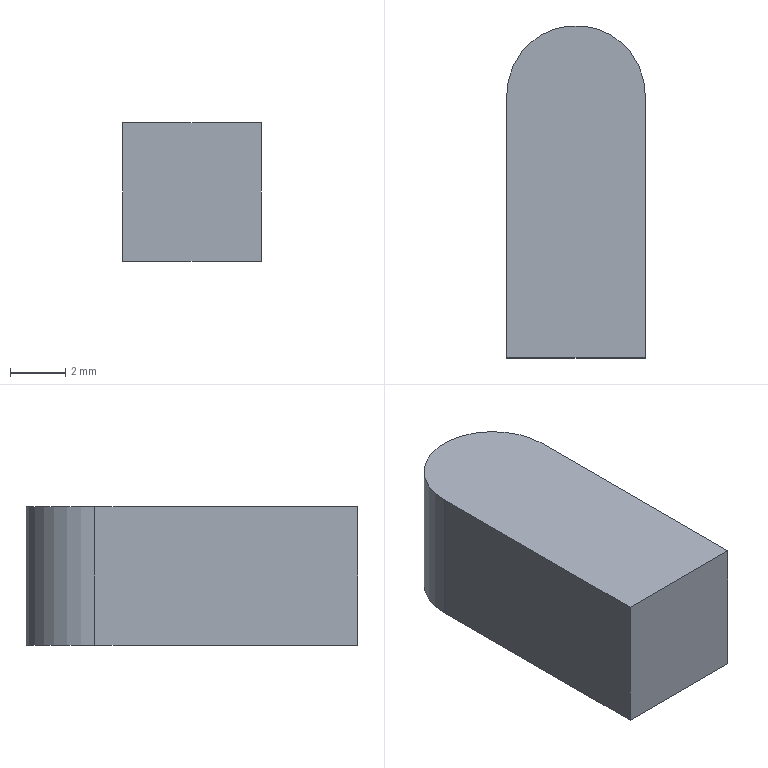Part | NX | features DATUM_CSYS 2, EXTRUDE 1, FACE_BLEND 1, SKETCH 1 | 1 solid | 6 faces | box 5 x 12 x 5 mm | volume 286.587 mm3 | plane 5 | cylinder 1 | commonest cylinder face diameters 5 x1
STEP:
#1=CARTESIAN_POINT('',(2.5,9.5,0.));
#2=VERTEX_POINT('',#1);
#3=CARTESIAN_POINT('',(2.5,9.5,5.));
#4=VERTEX_POINT('',#3);
#5=CARTESIAN_POINT('',(2.5,9.5,5.));
#6=DIRECTION('',(0.,0.,1.));
#7=VECTOR('',#6,1000.);
#8=LINE('',#5,#7);
#9=EDGE_CURVE('',#2,#4,#8,.T.);
#10=ORIENTED_EDGE('',*,*,#9,.F.);
#11=CARTESIAN_POINT('',(-2.5,9.5,0.));
#12=VERTEX_POINT('',#11);
#13=CARTESIAN_POINT('',(0.,9.5,0.));
#14=DIRECTION('',(0.,0.,1.));
#15=DIRECTION('',(1.,0.,0.));
#16=AXIS2_PLACEMENT_3D('',#13,#14,#15);
#17=CIRCLE('',#16,2.5);
#18=EDGE_CURVE('',#12,#2,#17,.F.);
#19=ORIENTED_EDGE('',*,*,#18,.F.);
#20=CARTESIAN_POINT('',(-2.5,9.5,5.));
#21=VERTEX_POINT('',#20);
#22=CARTESIAN_POINT('',(-2.5,9.5,5.));
#23=DIRECTION('',(0.,0.,1.));
#24=VECTOR('',#23,1000.);
#25=LINE('',#22,#24);
#26=EDGE_CURVE('',#21,#12,#25,.F.);
#27=ORIENTED_EDGE('',*,*,#26,.F.);
#28=CARTESIAN_POINT('',(0.,9.5,5.));
#29=DIRECTION('',(0.,0.,1.));
#30=DIRECTION('',(1.,0.,0.));
#31=AXIS2_PLACEMENT_3D('',#28,#29,#30);
#32=CIRCLE('',#31,2.5);
#33=EDGE_CURVE('',#4,#21,#32,.T.);
#34=ORIENTED_EDGE('',*,*,#33,.F.);
#35=EDGE_LOOP('',(#10,#19,#27,#34));
#36=FACE_BOUND('',#35,.T.);
#37=CARTESIAN_POINT('',(0.,9.5,0.));
#38=DIRECTION('',(0.,0.,1.));
#39=DIRECTION('',(1.,0.,0.));
#40=AXIS2_PLACEMENT_3D('',#37,#38,#39);
#41=CYLINDRICAL_SURFACE('',#40,2.5);
#42=ADVANCED_FACE('',(#36),#41,.T.);
#43=CARTESIAN_POINT('',(-2.5,0.,5.));
#44=VERTEX_POINT('',#43);
#45=CARTESIAN_POINT('',(-2.5,12.,5.));
#46=DIRECTION('',(0.,-1.,0.));
#47=VECTOR('',#46,1000.);
#48=LINE('',#45,#47);
#49=EDGE_CURVE('',#21,#44,#48,.T.);
#50=ORIENTED_EDGE('',*,*,#49,.F.);
#51=ORIENTED_EDGE('',*,*,#26,.T.);
#52=CARTESIAN_POINT('',(-2.5,0.,0.));
#53=VERTEX_POINT('',#52);
#54=CARTESIAN_POINT('',(-2.5,12.,0.));
#55=DIRECTION('',(0.,-1.,0.));
#56=VECTOR('',#55,1000.);
#57=LINE('',#54,#56);
#58=EDGE_CURVE('',#12,#53,#57,.T.);
#59=ORIENTED_EDGE('',*,*,#58,.T.);
#60=CARTESIAN_POINT('',(-2.5,0.,5.));
#61=DIRECTION('',(0.,0.,-1.));
#62=VECTOR('',#61,1000.);
#63=LINE('',#60,#62);
#64=EDGE_CURVE('',#44,#53,#63,.T.);
#65=ORIENTED_EDGE('',*,*,#64,.F.);
#66=EDGE_LOOP('',(#50,#51,#59,#65));
#67=FACE_BOUND('',#66,.T.);
#68=CARTESIAN_POINT('',(-2.5,12.,5.));
#69=DIRECTION('',(1.,0.,0.));
#70=DIRECTION('',(0.,1.,0.));
#71=AXIS2_PLACEMENT_3D('',#68,#69,#70);
#72=PLANE('',#71);
#73=ADVANCED_FACE('',(#67),#72,.F.);
#74=CARTESIAN_POINT('',(2.5,0.,0.));
#75=VERTEX_POINT('',#74);
#76=CARTESIAN_POINT('',(-2.5,0.,0.));
#77=DIRECTION('',(1.,0.,0.));
#78=VECTOR('',#77,1000.);
#79=LINE('',#76,#78);
#80=EDGE_CURVE('',#53,#75,#79,.T.);
#81=ORIENTED_EDGE('',*,*,#80,.T.);
#82=CARTESIAN_POINT('',(2.5,0.,5.));
#83=VERTEX_POINT('',#82);
#84=CARTESIAN_POINT('',(2.5,0.,5.));
#85=DIRECTION('',(0.,0.,-1.));
#86=VECTOR('',#85,1000.);
#87=LINE('',#84,#86);
#88=EDGE_CURVE('',#83,#75,#87,.T.);
#89=ORIENTED_EDGE('',*,*,#88,.F.);
#90=CARTESIAN_POINT('',(-2.5,0.,5.));
#91=DIRECTION('',(1.,0.,0.));
#92=VECTOR('',#91,1000.);
#93=LINE('',#90,#92);
#94=EDGE_CURVE('',#44,#83,#93,.T.);
#95=ORIENTED_EDGE('',*,*,#94,.F.);
#96=ORIENTED_EDGE('',*,*,#64,.T.);
#97=EDGE_LOOP('',(#81,#89,#95,#96));
#98=FACE_BOUND('',#97,.T.);
#99=CARTESIAN_POINT('',(-2.5,0.,5.));
#100=DIRECTION('',(0.,1.,0.));
#101=DIRECTION('',(0.,0.,1.));
#102=AXIS2_PLACEMENT_3D('',#99,#100,#101);
#103=PLANE('',#102);
#104=ADVANCED_FACE('',(#98),#103,.F.);
#105=CARTESIAN_POINT('',(2.5,0.,0.));
#106=DIRECTION('',(0.,1.,0.));
#107=VECTOR('',#106,1000.);
#108=LINE('',#105,#107);
#109=EDGE_CURVE('',#75,#2,#108,.T.);
#110=ORIENTED_EDGE('',*,*,#109,.T.);
#111=ORIENTED_EDGE('',*,*,#9,.T.);
#112=CARTESIAN_POINT('',(2.5,0.,5.));
#113=DIRECTION('',(0.,1.,0.));
#114=VECTOR('',#113,1000.);
#115=LINE('',#112,#114);
#116=EDGE_CURVE('',#83,#4,#115,.T.);
#117=ORIENTED_EDGE('',*,*,#116,.F.);
#118=ORIENTED_EDGE('',*,*,#88,.T.);
#119=EDGE_LOOP('',(#110,#111,#117,#118));
#120=FACE_BOUND('',#119,.T.);
#121=CARTESIAN_POINT('',(2.5,0.,5.));
#122=DIRECTION('',(-1.,0.,0.));
#123=DIRECTION('',(0.,-1.,0.));
#124=AXIS2_PLACEMENT_3D('',#121,#122,#123);
#125=PLANE('',#124);
#126=ADVANCED_FACE('',(#120),#125,.F.);
#127=ORIENTED_EDGE('',*,*,#116,.T.);
#128=ORIENTED_EDGE('',*,*,#33,.T.);
#129=ORIENTED_EDGE('',*,*,#49,.T.);
#130=ORIENTED_EDGE('',*,*,#94,.T.);
#131=EDGE_LOOP('',(#127,#128,#129,#130));
#132=FACE_BOUND('',#131,.T.);
#133=CARTESIAN_POINT('',(0.,0.,5.));
#134=DIRECTION('',(0.,0.,1.));
#135=DIRECTION('',(1.,0.,0.));
#136=AXIS2_PLACEMENT_3D('',#133,#134,#135);
#137=PLANE('',#136);
#138=ADVANCED_FACE('',(#132),#137,.T.);
#139=ORIENTED_EDGE('',*,*,#58,.F.);
#140=ORIENTED_EDGE('',*,*,#18,.T.);
#141=ORIENTED_EDGE('',*,*,#109,.F.);
#142=ORIENTED_EDGE('',*,*,#80,.F.);
#143=EDGE_LOOP('',(#139,#140,#141,#142));
#144=FACE_BOUND('',#143,.T.);
#145=CARTESIAN_POINT('',(0.,0.,0.));
#146=DIRECTION('',(0.,0.,1.));
#147=DIRECTION('',(1.,0.,0.));
#148=AXIS2_PLACEMENT_3D('',#145,#146,#147);
#149=PLANE('',#148);
#150=ADVANCED_FACE('',(#144),#149,.F.);
#151=CLOSED_SHELL('',(#42,#73,#104,#126,#138,#150));
#152=MANIFOLD_SOLID_BREP('',#151);
#153=(LENGTH_UNIT()NAMED_UNIT(*)SI_UNIT(.MILLI.,.METRE.));
#154=UNCERTAINTY_MEASURE_WITH_UNIT(LENGTH_MEASURE(0.00001),#153,'','');
#155=(NAMED_UNIT(*)PLANE_ANGLE_UNIT()SI_UNIT($,.RADIAN.));
#156=(NAMED_UNIT(*)SI_UNIT($,.STERADIAN.)SOLID_ANGLE_UNIT());
#157=(GEOMETRIC_REPRESENTATION_CONTEXT(3)GLOBAL_UNCERTAINTY_ASSIGNED_CONTEXT((#154))GLOBAL_UNIT_ASSIGNED_CONTEXT((#153,#155,#156))REPRESENTATION_CONTEXT('',''));
#158=ADVANCED_BREP_SHAPE_REPRESENTATION('',(#152),#157);